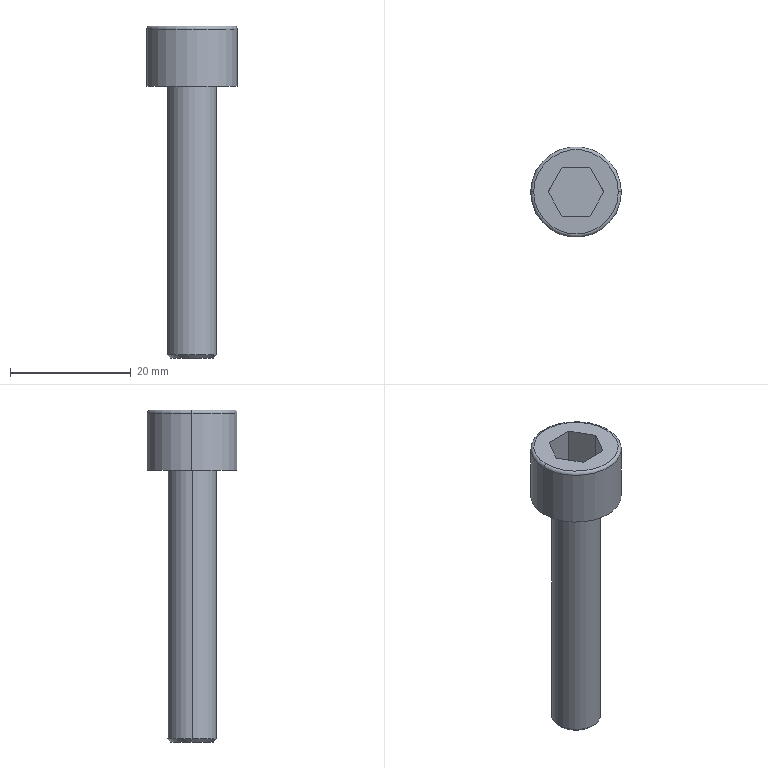Part | CATIA | 1 solid | 18 faces | box 15 x 15 x 55 mm | volume 3637 mm3 | plane 10 | cylinder 4 | torus 2 | cone 2 | commonest cylinder face diameters 8.1 x2 15 x2
STEP:
#1=CARTESIAN_POINT('',(-7.5,0.,0.));
#2=VERTEX_POINT('',#1);
#3=CARTESIAN_POINT('',(7.5,0.,0.));
#4=VERTEX_POINT('',#3);
#5=CARTESIAN_POINT('',(0.,0.,0.));
#6=DIRECTION('',(0.,0.,1.));
#7=AXIS2_PLACEMENT_3D('',#5,#6,$);
#8=CIRCLE('',#7,7.5);
#9=EDGE_CURVE('',#2,#4,#8,.T.);
#10=ORIENTED_EDGE('',*,*,#9,.F.);
#11=CARTESIAN_POINT('',(0.,0.,0.));
#12=DIRECTION('',(0.,0.,1.));
#13=AXIS2_PLACEMENT_3D('',#11,#12,$);
#14=CIRCLE('',#13,7.5);
#15=EDGE_CURVE('',#4,#2,#14,.T.);
#16=ORIENTED_EDGE('',*,*,#15,.F.);
#17=EDGE_LOOP('',(#10,#16));
#18=FACE_OUTER_BOUND('',#17,.T.);
#19=CARTESIAN_POINT('',(-4.05,0.,0.));
#20=VERTEX_POINT('',#19);
#21=CARTESIAN_POINT('',(4.05,0.,0.));
#22=VERTEX_POINT('',#21);
#23=CARTESIAN_POINT('',(0.,0.,0.));
#24=DIRECTION('',(0.,0.,1.));
#25=AXIS2_PLACEMENT_3D('',#23,#24,$);
#26=CIRCLE('',#25,4.05);
#27=EDGE_CURVE('',#20,#22,#26,.F.);
#28=ORIENTED_EDGE('',*,*,#27,.F.);
#29=CARTESIAN_POINT('',(0.,0.,0.));
#30=DIRECTION('',(0.,0.,1.));
#31=AXIS2_PLACEMENT_3D('',#29,#30,$);
#32=CIRCLE('',#31,4.05);
#33=EDGE_CURVE('',#22,#20,#32,.F.);
#34=ORIENTED_EDGE('',*,*,#33,.F.);
#35=EDGE_LOOP('',(#28,#34));
#36=FACE_BOUND('',#35,.T.);
#37=CARTESIAN_POINT('',(0.,0.,0.));
#38=DIRECTION('',(0.,0.,1.));
#39=DIRECTION('',(1.,0.,0.));
#40=AXIS2_PLACEMENT_3D('',#37,#38,#39);
#41=PLANE('',#40);
#42=ADVANCED_FACE('',(#18,#36),#41,.F.);
#43=CARTESIAN_POINT('',(-2.309,-4.,10.));
#44=VERTEX_POINT('',#43);
#45=CARTESIAN_POINT('',(-2.309,-4.,2.));
#46=VERTEX_POINT('',#45);
#47=CARTESIAN_POINT('',(-2.309,-4.,6.));
#48=DIRECTION('',(0.,0.,-1.));
#49=VECTOR('',#48,1.);
#50=LINE('',#47,#49);
#51=EDGE_CURVE('',#44,#46,#50,.T.);
#52=ORIENTED_EDGE('',*,*,#51,.F.);
#53=CARTESIAN_POINT('',(2.309,-4.,10.));
#54=VERTEX_POINT('',#53);
#55=CARTESIAN_POINT('',(0.,-4.,10.));
#56=DIRECTION('',(1.,0.,0.));
#57=VECTOR('',#56,1.);
#58=LINE('',#55,#57);
#59=EDGE_CURVE('',#44,#54,#58,.T.);
#60=ORIENTED_EDGE('',*,*,#59,.T.);
#61=CARTESIAN_POINT('',(2.309,-4.,2.));
#62=VERTEX_POINT('',#61);
#63=CARTESIAN_POINT('',(2.309,-4.,6.));
#64=DIRECTION('',(0.,0.,-1.));
#65=VECTOR('',#64,1.);
#66=LINE('',#63,#65);
#67=EDGE_CURVE('',#54,#62,#66,.T.);
#68=ORIENTED_EDGE('',*,*,#67,.T.);
#69=CARTESIAN_POINT('',(0.,-4.,2.));
#70=DIRECTION('',(1.,0.,0.));
#71=VECTOR('',#70,1.);
#72=LINE('',#69,#71);
#73=EDGE_CURVE('',#46,#62,#72,.T.);
#74=ORIENTED_EDGE('',*,*,#73,.F.);
#75=EDGE_LOOP('',(#52,#60,#68,#74));
#76=FACE_OUTER_BOUND('',#75,.T.);
#77=CARTESIAN_POINT('',(-2.309,-4.,10.));
#78=DIRECTION('',(0.,1.,0.));
#79=DIRECTION('',(1.,0.,0.));
#80=AXIS2_PLACEMENT_3D('',#77,#78,#79);
#81=PLANE('',#80);
#82=ADVANCED_FACE('',(#76),#81,.T.);
#83=CARTESIAN_POINT('',(-4.619,0.,10.));
#84=VERTEX_POINT('',#83);
#85=CARTESIAN_POINT('',(-4.619,0.,2.));
#86=VERTEX_POINT('',#85);
#87=CARTESIAN_POINT('',(-4.619,0.,6.));
#88=DIRECTION('',(0.,0.,-1.));
#89=VECTOR('',#88,1.);
#90=LINE('',#87,#89);
#91=EDGE_CURVE('',#84,#86,#90,.T.);
#92=ORIENTED_EDGE('',*,*,#91,.F.);
#93=CARTESIAN_POINT('',(-3.464,-2.,10.));
#94=DIRECTION('',(0.5,-0.866,0.));
#95=VECTOR('',#94,1.);
#96=LINE('',#93,#95);
#97=EDGE_CURVE('',#84,#44,#96,.T.);
#98=ORIENTED_EDGE('',*,*,#97,.T.);
#99=ORIENTED_EDGE('',*,*,#51,.T.);
#100=CARTESIAN_POINT('',(-3.464,-2.,2.));
#101=DIRECTION('',(0.5,-0.866,0.));
#102=VECTOR('',#101,1.);
#103=LINE('',#100,#102);
#104=EDGE_CURVE('',#86,#46,#103,.T.);
#105=ORIENTED_EDGE('',*,*,#104,.F.);
#106=EDGE_LOOP('',(#92,#98,#99,#105));
#107=FACE_OUTER_BOUND('',#106,.T.);
#108=CARTESIAN_POINT('',(-4.619,0.,10.));
#109=DIRECTION('',(0.866,0.5,0.));
#110=DIRECTION('',(0.5,-0.866,0.));
#111=AXIS2_PLACEMENT_3D('',#108,#109,#110);
#112=PLANE('',#111);
#113=ADVANCED_FACE('',(#107),#112,.T.);
#114=ORIENTED_EDGE('',*,*,#67,.F.);
#115=CARTESIAN_POINT('',(4.619,0.,10.));
#116=VERTEX_POINT('',#115);
#117=CARTESIAN_POINT('',(3.464,-2.,10.));
#118=DIRECTION('',(0.5,0.866,0.));
#119=VECTOR('',#118,1.);
#120=LINE('',#117,#119);
#121=EDGE_CURVE('',#54,#116,#120,.T.);
#122=ORIENTED_EDGE('',*,*,#121,.T.);
#123=CARTESIAN_POINT('',(4.619,0.,2.));
#124=VERTEX_POINT('',#123);
#125=CARTESIAN_POINT('',(4.619,0.,6.));
#126=DIRECTION('',(0.,0.,-1.));
#127=VECTOR('',#126,1.);
#128=LINE('',#125,#127);
#129=EDGE_CURVE('',#116,#124,#128,.T.);
#130=ORIENTED_EDGE('',*,*,#129,.T.);
#131=CARTESIAN_POINT('',(3.464,-2.,2.));
#132=DIRECTION('',(0.5,0.866,0.));
#133=VECTOR('',#132,1.);
#134=LINE('',#131,#133);
#135=EDGE_CURVE('',#62,#124,#134,.T.);
#136=ORIENTED_EDGE('',*,*,#135,.F.);
#137=EDGE_LOOP('',(#114,#122,#130,#136));
#138=FACE_OUTER_BOUND('',#137,.T.);
#139=CARTESIAN_POINT('',(2.309,-4.,10.));
#140=DIRECTION('',(-0.866,0.5,0.));
#141=DIRECTION('',(0.5,0.866,0.));
#142=AXIS2_PLACEMENT_3D('',#139,#140,#141);
#143=PLANE('',#142);
#144=ADVANCED_FACE('',(#138),#143,.T.);
#145=CARTESIAN_POINT('',(2.309,4.,2.));
#146=VERTEX_POINT('',#145);
#147=CARTESIAN_POINT('',(-2.309,4.,2.));
#148=VERTEX_POINT('',#147);
#149=CARTESIAN_POINT('',(0.,4.,2.));
#150=DIRECTION('',(-1.,0.,0.));
#151=VECTOR('',#150,1.);
#152=LINE('',#149,#151);
#153=EDGE_CURVE('',#146,#148,#152,.T.);
#154=ORIENTED_EDGE('',*,*,#153,.T.);
#155=CARTESIAN_POINT('',(-3.464,2.,2.));
#156=DIRECTION('',(-0.5,-0.866,0.));
#157=VECTOR('',#156,1.);
#158=LINE('',#155,#157);
#159=EDGE_CURVE('',#148,#86,#158,.T.);
#160=ORIENTED_EDGE('',*,*,#159,.T.);
#161=ORIENTED_EDGE('',*,*,#104,.T.);
#162=ORIENTED_EDGE('',*,*,#73,.T.);
#163=ORIENTED_EDGE('',*,*,#135,.T.);
#164=CARTESIAN_POINT('',(3.464,2.,2.));
#165=DIRECTION('',(-0.5,0.866,0.));
#166=VECTOR('',#165,1.);
#167=LINE('',#164,#166);
#168=EDGE_CURVE('',#124,#146,#167,.T.);
#169=ORIENTED_EDGE('',*,*,#168,.T.);
#170=EDGE_LOOP('',(#154,#160,#161,#162,#163,#169));
#171=FACE_OUTER_BOUND('',#170,.T.);
#172=CARTESIAN_POINT('',(0.,0.,2.));
#173=DIRECTION('',(0.,0.,1.));
#174=DIRECTION('',(1.,0.,0.));
#175=AXIS2_PLACEMENT_3D('',#172,#173,#174);
#176=PLANE('',#175);
#177=ADVANCED_FACE('',(#171),#176,.T.);
#178=CARTESIAN_POINT('',(-2.309,4.,10.));
#179=VERTEX_POINT('',#178);
#180=CARTESIAN_POINT('',(-2.309,4.,6.));
#181=DIRECTION('',(0.,0.,-1.));
#182=VECTOR('',#181,1.);
#183=LINE('',#180,#182);
#184=EDGE_CURVE('',#179,#148,#183,.T.);
#185=ORIENTED_EDGE('',*,*,#184,.F.);
#186=CARTESIAN_POINT('',(-3.464,2.,10.));
#187=DIRECTION('',(-0.5,-0.866,0.));
#188=VECTOR('',#187,1.);
#189=LINE('',#186,#188);
#190=EDGE_CURVE('',#179,#84,#189,.T.);
#191=ORIENTED_EDGE('',*,*,#190,.T.);
#192=ORIENTED_EDGE('',*,*,#91,.T.);
#193=ORIENTED_EDGE('',*,*,#159,.F.);
#194=EDGE_LOOP('',(#185,#191,#192,#193));
#195=FACE_OUTER_BOUND('',#194,.T.);
#196=CARTESIAN_POINT('',(-2.309,4.,10.));
#197=DIRECTION('',(0.866,-0.5,0.));
#198=DIRECTION('',(-0.5,-0.866,0.));
#199=AXIS2_PLACEMENT_3D('',#196,#197,#198);
#200=PLANE('',#199);
#201=ADVANCED_FACE('',(#195),#200,.T.);
#202=ORIENTED_EDGE('',*,*,#129,.F.);
#203=CARTESIAN_POINT('',(2.309,4.,10.));
#204=VERTEX_POINT('',#203);
#205=CARTESIAN_POINT('',(3.464,2.,10.));
#206=DIRECTION('',(-0.5,0.866,0.));
#207=VECTOR('',#206,1.);
#208=LINE('',#205,#207);
#209=EDGE_CURVE('',#116,#204,#208,.T.);
#210=ORIENTED_EDGE('',*,*,#209,.T.);
#211=CARTESIAN_POINT('',(2.309,4.,6.));
#212=DIRECTION('',(0.,0.,-1.));
#213=VECTOR('',#212,1.);
#214=LINE('',#211,#213);
#215=EDGE_CURVE('',#204,#146,#214,.T.);
#216=ORIENTED_EDGE('',*,*,#215,.T.);
#217=ORIENTED_EDGE('',*,*,#168,.F.);
#218=EDGE_LOOP('',(#202,#210,#216,#217));
#219=FACE_OUTER_BOUND('',#218,.T.);
#220=CARTESIAN_POINT('',(4.619,0.,10.));
#221=DIRECTION('',(-0.866,-0.5,0.));
#222=DIRECTION('',(-0.5,0.866,0.));
#223=AXIS2_PLACEMENT_3D('',#220,#221,#222);
#224=PLANE('',#223);
#225=ADVANCED_FACE('',(#219),#224,.T.);
#226=ORIENTED_EDGE('',*,*,#215,.F.);
#227=CARTESIAN_POINT('',(0.,4.,10.));
#228=DIRECTION('',(-1.,0.,0.));
#229=VECTOR('',#228,1.);
#230=LINE('',#227,#229);
#231=EDGE_CURVE('',#204,#179,#230,.T.);
#232=ORIENTED_EDGE('',*,*,#231,.T.);
#233=ORIENTED_EDGE('',*,*,#184,.T.);
#234=ORIENTED_EDGE('',*,*,#153,.F.);
#235=EDGE_LOOP('',(#226,#232,#233,#234));
#236=FACE_OUTER_BOUND('',#235,.T.);
#237=CARTESIAN_POINT('',(2.309,4.,10.));
#238=DIRECTION('',(0.,-1.,0.));
#239=DIRECTION('',(-1.,0.,0.));
#240=AXIS2_PLACEMENT_3D('',#237,#238,#239);
#241=PLANE('',#240);
#242=ADVANCED_FACE('',(#236),#241,.T.);
#243=CARTESIAN_POINT('',(-7.,0.000000007,10.));
#244=VERTEX_POINT('',#243);
#245=CARTESIAN_POINT('',(7.,0.,10.));
#246=VERTEX_POINT('',#245);
#247=CARTESIAN_POINT('',(0.,0.,10.));
#248=DIRECTION('',(0.,0.,1.));
#249=AXIS2_PLACEMENT_3D('',#247,#248,$);
#250=CIRCLE('',#249,7.);
#251=EDGE_CURVE('',#244,#246,#250,.T.);
#252=ORIENTED_EDGE('',*,*,#251,.T.);
#253=CARTESIAN_POINT('',(0.,0.,10.));
#254=DIRECTION('',(0.,0.,1.));
#255=AXIS2_PLACEMENT_3D('',#253,#254,$);
#256=CIRCLE('',#255,7.);
#257=EDGE_CURVE('',#246,#244,#256,.T.);
#258=ORIENTED_EDGE('',*,*,#257,.T.);
#259=EDGE_LOOP('',(#252,#258));
#260=FACE_OUTER_BOUND('',#259,.T.);
#261=ORIENTED_EDGE('',*,*,#121,.F.);
#262=ORIENTED_EDGE('',*,*,#59,.F.);
#263=ORIENTED_EDGE('',*,*,#97,.F.);
#264=ORIENTED_EDGE('',*,*,#190,.F.);
#265=ORIENTED_EDGE('',*,*,#231,.F.);
#266=ORIENTED_EDGE('',*,*,#209,.F.);
#267=EDGE_LOOP('',(#261,#262,#263,#264,#265,#266));
#268=FACE_BOUND('',#267,.T.);
#269=CARTESIAN_POINT('',(0.,0.,10.));
#270=DIRECTION('',(0.,0.,1.));
#271=DIRECTION('',(1.,0.,0.));
#272=AXIS2_PLACEMENT_3D('',#269,#270,#271);
#273=PLANE('',#272);
#274=ADVANCED_FACE('',(#260,#268),#273,.T.);
#275=CARTESIAN_POINT('',(-7.5,0.,9.5));
#276=VERTEX_POINT('',#275);
#277=CARTESIAN_POINT('',(-7.5,0.,5.));
#278=DIRECTION('',(0.,0.,1.));
#279=VECTOR('',#278,1.);
#280=LINE('',#277,#279);
#281=EDGE_CURVE('',#2,#276,#280,.T.);
#282=ORIENTED_EDGE('',*,*,#281,.F.);
#283=ORIENTED_EDGE('',*,*,#9,.T.);
#284=CARTESIAN_POINT('',(7.5,0.,9.5));
#285=VERTEX_POINT('',#284);
#286=CARTESIAN_POINT('',(7.5,0.,5.));
#287=DIRECTION('',(0.,0.,1.));
#288=VECTOR('',#287,1.);
#289=LINE('',#286,#288);
#290=EDGE_CURVE('',#4,#285,#289,.T.);
#291=ORIENTED_EDGE('',*,*,#290,.T.);
#292=CARTESIAN_POINT('',(0.,0.,9.5));
#293=DIRECTION('',(0.,0.,1.));
#294=AXIS2_PLACEMENT_3D('',#292,#293,$);
#295=CIRCLE('',#294,7.5);
#296=EDGE_CURVE('',#276,#285,#295,.T.);
#297=ORIENTED_EDGE('',*,*,#296,.F.);
#298=EDGE_LOOP('',(#282,#283,#291,#297));
#299=FACE_OUTER_BOUND('',#298,.T.);
#300=CARTESIAN_POINT('',(0.,0.,5.));
#301=DIRECTION('',(0.,0.,1.));
#302=DIRECTION('',(1.,0.,0.));
#303=AXIS2_PLACEMENT_3D('',#300,#301,#302);
#304=CYLINDRICAL_SURFACE('',#303,7.5);
#305=ADVANCED_FACE('',(#299),#304,.T.);
#306=ORIENTED_EDGE('',*,*,#290,.F.);
#307=ORIENTED_EDGE('',*,*,#15,.T.);
#308=ORIENTED_EDGE('',*,*,#281,.T.);
#309=CARTESIAN_POINT('',(0.,0.,9.5));
#310=DIRECTION('',(0.,0.,1.));
#311=AXIS2_PLACEMENT_3D('',#309,#310,$);
#312=CIRCLE('',#311,7.5);
#313=EDGE_CURVE('',#285,#276,#312,.T.);
#314=ORIENTED_EDGE('',*,*,#313,.F.);
#315=EDGE_LOOP('',(#306,#307,#308,#314));
#316=FACE_OUTER_BOUND('',#315,.T.);
#317=ADVANCED_FACE('',(#316),#304,.T.);
#318=CARTESIAN_POINT('',(-7.,0.,9.5));
#319=DIRECTION('',(0.,1.,0.));
#320=AXIS2_PLACEMENT_3D('',#318,#319,$);
#321=CIRCLE('',#320,0.5);
#322=EDGE_CURVE('',#244,#276,#321,.F.);
#323=ORIENTED_EDGE('',*,*,#322,.T.);
#324=ORIENTED_EDGE('',*,*,#296,.T.);
#325=CARTESIAN_POINT('',(7.,0.,9.5));
#326=DIRECTION('',(0.,-1.,0.));
#327=AXIS2_PLACEMENT_3D('',#325,#326,$);
#328=CIRCLE('',#327,0.5);
#329=EDGE_CURVE('',#246,#285,#328,.F.);
#330=ORIENTED_EDGE('',*,*,#329,.F.);
#331=ORIENTED_EDGE('',*,*,#251,.F.);
#332=EDGE_LOOP('',(#323,#324,#330,#331));
#333=FACE_OUTER_BOUND('',#332,.T.);
#334=CARTESIAN_POINT('',(0.,0.,9.5));
#335=DIRECTION('',(0.,0.,1.));
#336=DIRECTION('',(-0.9999,0.01112,0.));
#337=AXIS2_PLACEMENT_3D('',#334,#335,#336);
#338=TOROIDAL_SURFACE('',#337,7.,0.5);
#339=ADVANCED_FACE('',(#333),#338,.T.);
#340=ORIENTED_EDGE('',*,*,#329,.T.);
#341=ORIENTED_EDGE('',*,*,#313,.T.);
#342=ORIENTED_EDGE('',*,*,#322,.F.);
#343=ORIENTED_EDGE('',*,*,#257,.F.);
#344=EDGE_LOOP('',(#340,#341,#342,#343));
#345=FACE_OUTER_BOUND('',#344,.T.);
#346=CARTESIAN_POINT('',(0.,0.,9.5));
#347=DIRECTION('',(0.,0.,1.));
#348=DIRECTION('',(1.,0.,0.));
#349=AXIS2_PLACEMENT_3D('',#346,#347,#348);
#350=TOROIDAL_SURFACE('',#349,7.,0.5);
#351=ADVANCED_FACE('',(#345),#350,.T.);
#352=CARTESIAN_POINT('',(4.05,0.,-44.5));
#353=VERTEX_POINT('',#352);
#354=CARTESIAN_POINT('',(4.05,0.,-22.5));
#355=DIRECTION('',(0.,0.,-1.));
#356=VECTOR('',#355,1.);
#357=LINE('',#354,#356);
#358=EDGE_CURVE('',#22,#353,#357,.T.);
#359=ORIENTED_EDGE('',*,*,#358,.F.);
#360=ORIENTED_EDGE('',*,*,#33,.T.);
#361=CARTESIAN_POINT('',(-4.05,0.,-44.5));
#362=VERTEX_POINT('',#361);
#363=CARTESIAN_POINT('',(-4.05,0.,-22.5));
#364=DIRECTION('',(0.,0.,-1.));
#365=VECTOR('',#364,1.);
#366=LINE('',#363,#365);
#367=EDGE_CURVE('',#20,#362,#366,.T.);
#368=ORIENTED_EDGE('',*,*,#367,.T.);
#369=CARTESIAN_POINT('',(0.,0.,-44.5));
#370=DIRECTION('',(0.,0.,-1.));
#371=AXIS2_PLACEMENT_3D('',#369,#370,$);
#372=CIRCLE('',#371,4.05);
#373=EDGE_CURVE('',#353,#362,#372,.T.);
#374=ORIENTED_EDGE('',*,*,#373,.F.);
#375=EDGE_LOOP('',(#359,#360,#368,#374));
#376=FACE_OUTER_BOUND('',#375,.T.);
#377=CARTESIAN_POINT('',(0.,0.,-22.5));
#378=DIRECTION('',(0.,0.,-1.));
#379=DIRECTION('',(1.,0.,0.));
#380=AXIS2_PLACEMENT_3D('',#377,#378,#379);
#381=CYLINDRICAL_SURFACE('',#380,4.05);
#382=ADVANCED_FACE('',(#376),#381,.T.);
#383=ORIENTED_EDGE('',*,*,#367,.F.);
#384=ORIENTED_EDGE('',*,*,#27,.T.);
#385=ORIENTED_EDGE('',*,*,#358,.T.);
#386=CARTESIAN_POINT('',(0.,0.,-44.5));
#387=DIRECTION('',(0.,0.,-1.));
#388=AXIS2_PLACEMENT_3D('',#386,#387,$);
#389=CIRCLE('',#388,4.05);
#390=EDGE_CURVE('',#362,#353,#389,.T.);
#391=ORIENTED_EDGE('',*,*,#390,.F.);
#392=EDGE_LOOP('',(#383,#384,#385,#391));
#393=FACE_OUTER_BOUND('',#392,.T.);
#394=ADVANCED_FACE('',(#393),#381,.T.);
#395=CARTESIAN_POINT('',(-3.55,-0.000000315,-45.));
#396=VERTEX_POINT('',#395);
#397=CARTESIAN_POINT('',(3.55,0.,-45.));
#398=VERTEX_POINT('',#397);
#399=CARTESIAN_POINT('',(0.,0.,-45.));
#400=DIRECTION('',(0.,0.,-1.));
#401=AXIS2_PLACEMENT_3D('',#399,#400,$);
#402=CIRCLE('',#401,3.55);
#403=EDGE_CURVE('',#396,#398,#402,.T.);
#404=ORIENTED_EDGE('',*,*,#403,.T.);
#405=CARTESIAN_POINT('',(0.,0.,-45.));
#406=DIRECTION('',(0.,0.,-1.));
#407=AXIS2_PLACEMENT_3D('',#405,#406,$);
#408=CIRCLE('',#407,3.55);
#409=EDGE_CURVE('',#398,#396,#408,.T.);
#410=ORIENTED_EDGE('',*,*,#409,.T.);
#411=EDGE_LOOP('',(#404,#410));
#412=FACE_OUTER_BOUND('',#411,.T.);
#413=CARTESIAN_POINT('',(0.,0.,-45.));
#414=DIRECTION('',(0.,0.,-1.));
#415=DIRECTION('',(1.,0.,0.));
#416=AXIS2_PLACEMENT_3D('',#413,#414,#415);
#417=PLANE('',#416);
#418=ADVANCED_FACE('',(#412),#417,.T.);
#419=CARTESIAN_POINT('',(-3.8,0.,-44.75));
#420=DIRECTION('',(-0.7071,0.,0.7071));
#421=VECTOR('',#420,1.);
#422=LINE('',#419,#421);
#423=EDGE_CURVE('',#396,#362,#422,.T.);
#424=ORIENTED_EDGE('',*,*,#423,.T.);
#425=ORIENTED_EDGE('',*,*,#390,.T.);
#426=CARTESIAN_POINT('',(3.8,0.,-44.75));
#427=DIRECTION('',(0.7071,0.,0.7071));
#428=VECTOR('',#427,1.);
#429=LINE('',#426,#428);
#430=EDGE_CURVE('',#398,#353,#429,.T.);
#431=ORIENTED_EDGE('',*,*,#430,.F.);
#432=ORIENTED_EDGE('',*,*,#403,.F.);
#433=EDGE_LOOP('',(#424,#425,#431,#432));
#434=FACE_OUTER_BOUND('',#433,.T.);
#435=CARTESIAN_POINT('',(0.,0.,-48.55));
#436=DIRECTION('',(0.,0.,1.));
#437=DIRECTION('',(-0.8191,-0.5736,0.));
#438=AXIS2_PLACEMENT_3D('',#435,#436,#437);
#439=CONICAL_SURFACE('',#438,0.,0.7854);
#440=ADVANCED_FACE('',(#434),#439,.T.);
#441=ORIENTED_EDGE('',*,*,#430,.T.);
#442=ORIENTED_EDGE('',*,*,#373,.T.);
#443=ORIENTED_EDGE('',*,*,#423,.F.);
#444=ORIENTED_EDGE('',*,*,#409,.F.);
#445=EDGE_LOOP('',(#441,#442,#443,#444));
#446=FACE_OUTER_BOUND('',#445,.T.);
#447=CARTESIAN_POINT('',(0.,0.,-48.55));
#448=DIRECTION('',(0.,0.,1.));
#449=DIRECTION('',(1.,0.,0.));
#450=AXIS2_PLACEMENT_3D('',#447,#448,#449);
#451=CONICAL_SURFACE('',#450,0.,0.7854);
#452=ADVANCED_FACE('',(#446),#451,.T.);
#453=CLOSED_SHELL('',(#42,#82,#113,#144,#177,#201,#225,#242,#274,#305,#317,#339,#351,#382,#394,#418,#440,#452));
#454=MANIFOLD_SOLID_BREP('',#453);
#455=(LENGTH_UNIT()NAMED_UNIT(*)SI_UNIT(.MILLI.,.METRE.));
#456=UNCERTAINTY_MEASURE_WITH_UNIT(LENGTH_MEASURE(0.005),#455,'','');
#457=(NAMED_UNIT(*)PLANE_ANGLE_UNIT()SI_UNIT($,.RADIAN.));
#458=(NAMED_UNIT(*)SI_UNIT($,.STERADIAN.)SOLID_ANGLE_UNIT());
#459=(GEOMETRIC_REPRESENTATION_CONTEXT(3)GLOBAL_UNCERTAINTY_ASSIGNED_CONTEXT((#456))GLOBAL_UNIT_ASSIGNED_CONTEXT((#455,#457,#458))REPRESENTATION_CONTEXT('',''));
#460=ADVANCED_BREP_SHAPE_REPRESENTATION('',(#454),#459);